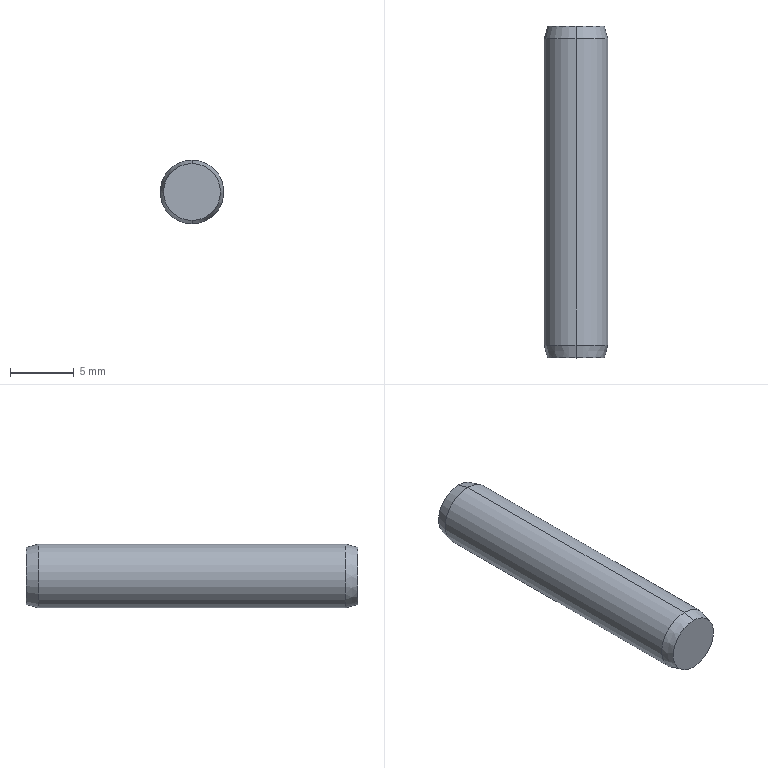Part | SolidWorks | features Chamfer 2, Extrusion 1 | 1 solid | 8 faces | box 5 x 26 x 5 mm | volume 506.42 mm3 | cone 4 | cylinder 2 | plane 2 | commonest cylinder face diameters 5 x2
STEP:
#1=CARTESIAN_POINT('',(0.,-13.,-2.23));
#2=VERTEX_POINT('',#1);
#3=CARTESIAN_POINT('',(0.,-13.,2.23));
#4=VERTEX_POINT('',#3);
#5=CARTESIAN_POINT('',(0.,-13.,0.));
#6=DIRECTION('',(0.,-1.,0.));
#7=DIRECTION('',(0.,0.,1.));
#8=AXIS2_PLACEMENT_3D('',#5,#6,#7);
#9=CIRCLE('',#8,2.23);
#10=EDGE_CURVE('',#2,#4,#9,.T.);
#11=ORIENTED_EDGE('',*,*,#10,.F.);
#12=CARTESIAN_POINT('',(0.,-11.992,-2.5));
#13=VERTEX_POINT('',#12);
#14=CARTESIAN_POINT('',(0.,-11.992,-2.5));
#15=DIRECTION('',(0.,0.9659,-0.2588));
#16=VECTOR('',#15,1000.);
#17=LINE('',#14,#16);
#18=EDGE_CURVE('',#2,#13,#17,.T.);
#19=ORIENTED_EDGE('',*,*,#18,.T.);
#20=CARTESIAN_POINT('',(0.,-11.992,2.5));
#21=VERTEX_POINT('',#20);
#22=CARTESIAN_POINT('',(0.,-11.992,0.));
#23=DIRECTION('',(0.,1.,0.));
#24=DIRECTION('',(0.,0.,1.));
#25=AXIS2_PLACEMENT_3D('',#22,#23,#24);
#26=CIRCLE('',#25,2.5);
#27=EDGE_CURVE('',#21,#13,#26,.T.);
#28=ORIENTED_EDGE('',*,*,#27,.F.);
#29=CARTESIAN_POINT('',(0.,-11.992,2.5));
#30=DIRECTION('',(0.,0.9659,0.2588));
#31=VECTOR('',#30,1000.);
#32=LINE('',#29,#31);
#33=EDGE_CURVE('',#4,#21,#32,.T.);
#34=ORIENTED_EDGE('',*,*,#33,.F.);
#35=EDGE_LOOP('',(#11,#19,#28,#34));
#36=FACE_OUTER_BOUND('',#35,.T.);
#37=CARTESIAN_POINT('',(0.,-11.992,0.));
#38=DIRECTION('',(0.,1.,0.));
#39=DIRECTION('',(0.,0.,1.));
#40=AXIS2_PLACEMENT_3D('',#37,#38,#39);
#41=CONICAL_SURFACE('',#40,2.5,0.2618);
#42=ADVANCED_FACE('',(#36),#41,.T.);
#43=CARTESIAN_POINT('',(0.,13.,2.232));
#44=VERTEX_POINT('',#43);
#45=CARTESIAN_POINT('',(0.,13.,-2.232));
#46=VERTEX_POINT('',#45);
#47=CARTESIAN_POINT('',(0.,13.,0.));
#48=DIRECTION('',(0.,1.,0.));
#49=DIRECTION('',(0.,0.,1.));
#50=AXIS2_PLACEMENT_3D('',#47,#48,#49);
#51=CIRCLE('',#50,2.232);
#52=EDGE_CURVE('',#44,#46,#51,.T.);
#53=ORIENTED_EDGE('',*,*,#52,.F.);
#54=CARTESIAN_POINT('',(0.,12.,2.5));
#55=VERTEX_POINT('',#54);
#56=CARTESIAN_POINT('',(0.,13.,2.232));
#57=DIRECTION('',(0.,-0.9659,0.2588));
#58=VECTOR('',#57,1000.);
#59=LINE('',#56,#58);
#60=EDGE_CURVE('',#44,#55,#59,.T.);
#61=ORIENTED_EDGE('',*,*,#60,.T.);
#62=CARTESIAN_POINT('',(0.,12.,-2.5));
#63=VERTEX_POINT('',#62);
#64=CARTESIAN_POINT('',(0.,12.,0.));
#65=DIRECTION('',(0.,-1.,0.));
#66=DIRECTION('',(0.,0.,1.));
#67=AXIS2_PLACEMENT_3D('',#64,#65,#66);
#68=CIRCLE('',#67,2.5);
#69=EDGE_CURVE('',#63,#55,#68,.T.);
#70=ORIENTED_EDGE('',*,*,#69,.F.);
#71=CARTESIAN_POINT('',(0.,13.,-2.232));
#72=DIRECTION('',(0.,-0.9659,-0.2588));
#73=VECTOR('',#72,1000.);
#74=LINE('',#71,#73);
#75=EDGE_CURVE('',#46,#63,#74,.T.);
#76=ORIENTED_EDGE('',*,*,#75,.F.);
#77=EDGE_LOOP('',(#53,#61,#70,#76));
#78=FACE_OUTER_BOUND('',#77,.T.);
#79=CARTESIAN_POINT('',(0.,13.,0.));
#80=DIRECTION('',(0.,-1.,0.));
#81=DIRECTION('',(0.,0.,-1.));
#82=AXIS2_PLACEMENT_3D('',#79,#80,#81);
#83=CONICAL_SURFACE('',#82,2.232,0.2618);
#84=ADVANCED_FACE('',(#78),#83,.T.);
#85=ORIENTED_EDGE('',*,*,#69,.T.);
#86=CARTESIAN_POINT('',(0.,13.,2.5));
#87=DIRECTION('',(0.,-1.,0.));
#88=VECTOR('',#87,1000.);
#89=LINE('',#86,#88);
#90=EDGE_CURVE('',#55,#21,#89,.T.);
#91=ORIENTED_EDGE('',*,*,#90,.T.);
#92=ORIENTED_EDGE('',*,*,#27,.T.);
#93=CARTESIAN_POINT('',(0.,13.,-2.5));
#94=DIRECTION('',(0.,-1.,0.));
#95=VECTOR('',#94,1000.);
#96=LINE('',#93,#95);
#97=EDGE_CURVE('',#63,#13,#96,.T.);
#98=ORIENTED_EDGE('',*,*,#97,.F.);
#99=EDGE_LOOP('',(#85,#91,#92,#98));
#100=FACE_OUTER_BOUND('',#99,.T.);
#101=CARTESIAN_POINT('',(0.,13.,0.));
#102=DIRECTION('',(0.,-1.,0.));
#103=DIRECTION('',(0.,0.,-1.));
#104=AXIS2_PLACEMENT_3D('',#101,#102,#103);
#105=CYLINDRICAL_SURFACE('',#104,2.5);
#106=ADVANCED_FACE('',(#100),#105,.T.);
#107=ORIENTED_EDGE('',*,*,#90,.F.);
#108=CARTESIAN_POINT('',(0.,12.,0.));
#109=DIRECTION('',(0.,-1.,0.));
#110=DIRECTION('',(0.,0.,1.));
#111=AXIS2_PLACEMENT_3D('',#108,#109,#110);
#112=CIRCLE('',#111,2.5);
#113=EDGE_CURVE('',#55,#63,#112,.T.);
#114=ORIENTED_EDGE('',*,*,#113,.T.);
#115=ORIENTED_EDGE('',*,*,#97,.T.);
#116=CARTESIAN_POINT('',(0.,-11.992,0.));
#117=DIRECTION('',(0.,1.,0.));
#118=DIRECTION('',(0.,0.,1.));
#119=AXIS2_PLACEMENT_3D('',#116,#117,#118);
#120=CIRCLE('',#119,2.5);
#121=EDGE_CURVE('',#13,#21,#120,.T.);
#122=ORIENTED_EDGE('',*,*,#121,.T.);
#123=EDGE_LOOP('',(#107,#114,#115,#122));
#124=FACE_OUTER_BOUND('',#123,.T.);
#125=CARTESIAN_POINT('',(0.,13.,0.));
#126=DIRECTION('',(0.,-1.,0.));
#127=DIRECTION('',(0.,0.,-1.));
#128=AXIS2_PLACEMENT_3D('',#125,#126,#127);
#129=CYLINDRICAL_SURFACE('',#128,2.5);
#130=ADVANCED_FACE('',(#124),#129,.T.);
#131=CARTESIAN_POINT('',(0.,13.,0.));
#132=DIRECTION('',(0.,1.,0.));
#133=DIRECTION('',(0.,0.,1.));
#134=AXIS2_PLACEMENT_3D('',#131,#132,#133);
#135=CIRCLE('',#134,2.232);
#136=EDGE_CURVE('',#46,#44,#135,.T.);
#137=ORIENTED_EDGE('',*,*,#136,.T.);
#138=ORIENTED_EDGE('',*,*,#52,.T.);
#139=EDGE_LOOP('',(#137,#138));
#140=FACE_OUTER_BOUND('',#139,.T.);
#141=CARTESIAN_POINT('',(0.,13.,0.));
#142=DIRECTION('',(0.,1.,0.));
#143=DIRECTION('',(0.,0.,1.));
#144=AXIS2_PLACEMENT_3D('',#141,#142,#143);
#145=PLANE('',#144);
#146=ADVANCED_FACE('',(#140),#145,.T.);
#147=CARTESIAN_POINT('',(0.,-13.,0.));
#148=DIRECTION('',(0.,-1.,0.));
#149=DIRECTION('',(0.,0.,1.));
#150=AXIS2_PLACEMENT_3D('',#147,#148,#149);
#151=CIRCLE('',#150,2.23);
#152=EDGE_CURVE('',#4,#2,#151,.T.);
#153=ORIENTED_EDGE('',*,*,#152,.T.);
#154=ORIENTED_EDGE('',*,*,#10,.T.);
#155=EDGE_LOOP('',(#153,#154));
#156=FACE_OUTER_BOUND('',#155,.T.);
#157=CARTESIAN_POINT('',(0.,-13.,0.));
#158=DIRECTION('',(0.,1.,0.));
#159=DIRECTION('',(0.,0.,1.));
#160=AXIS2_PLACEMENT_3D('',#157,#158,#159);
#161=PLANE('',#160);
#162=ADVANCED_FACE('',(#156),#161,.F.);
#163=ORIENTED_EDGE('',*,*,#60,.F.);
#164=ORIENTED_EDGE('',*,*,#136,.F.);
#165=ORIENTED_EDGE('',*,*,#75,.T.);
#166=ORIENTED_EDGE('',*,*,#113,.F.);
#167=EDGE_LOOP('',(#163,#164,#165,#166));
#168=FACE_OUTER_BOUND('',#167,.T.);
#169=CARTESIAN_POINT('',(0.,13.,0.));
#170=DIRECTION('',(0.,-1.,0.));
#171=DIRECTION('',(0.,0.,-1.));
#172=AXIS2_PLACEMENT_3D('',#169,#170,#171);
#173=CONICAL_SURFACE('',#172,2.232,0.2618);
#174=ADVANCED_FACE('',(#168),#173,.T.);
#175=ORIENTED_EDGE('',*,*,#18,.F.);
#176=ORIENTED_EDGE('',*,*,#152,.F.);
#177=ORIENTED_EDGE('',*,*,#33,.T.);
#178=ORIENTED_EDGE('',*,*,#121,.F.);
#179=EDGE_LOOP('',(#175,#176,#177,#178));
#180=FACE_OUTER_BOUND('',#179,.T.);
#181=CARTESIAN_POINT('',(0.,-11.992,0.));
#182=DIRECTION('',(0.,1.,0.));
#183=DIRECTION('',(0.,0.,1.));
#184=AXIS2_PLACEMENT_3D('',#181,#182,#183);
#185=CONICAL_SURFACE('',#184,2.5,0.2618);
#186=ADVANCED_FACE('',(#180),#185,.T.);
#187=CLOSED_SHELL('',(#42,#84,#106,#130,#146,#162,#174,#186));
#188=MANIFOLD_SOLID_BREP('',#187);
#189=CARTESIAN_POINT('',(0.,0.,0.));
#190=DIRECTION('',(0.,0.,1.));
#191=DIRECTION('',(1.,0.,0.));
#192=AXIS2_PLACEMENT_3D('',#189,#190,#191);
#193=(LENGTH_UNIT()NAMED_UNIT(*)SI_UNIT(.MILLI.,.METRE.));
#194=UNCERTAINTY_MEASURE_WITH_UNIT(LENGTH_MEASURE(0.00001),#193,'','');
#195=(NAMED_UNIT(*)PLANE_ANGLE_UNIT()SI_UNIT($,.RADIAN.));
#196=(NAMED_UNIT(*)SI_UNIT($,.STERADIAN.)SOLID_ANGLE_UNIT());
#197=(GEOMETRIC_REPRESENTATION_CONTEXT(3)GLOBAL_UNCERTAINTY_ASSIGNED_CONTEXT((#194))GLOBAL_UNIT_ASSIGNED_CONTEXT((#193,#195,#196))REPRESENTATION_CONTEXT('',''));
#198=ADVANCED_BREP_SHAPE_REPRESENTATION('',(#188,#192),#197);